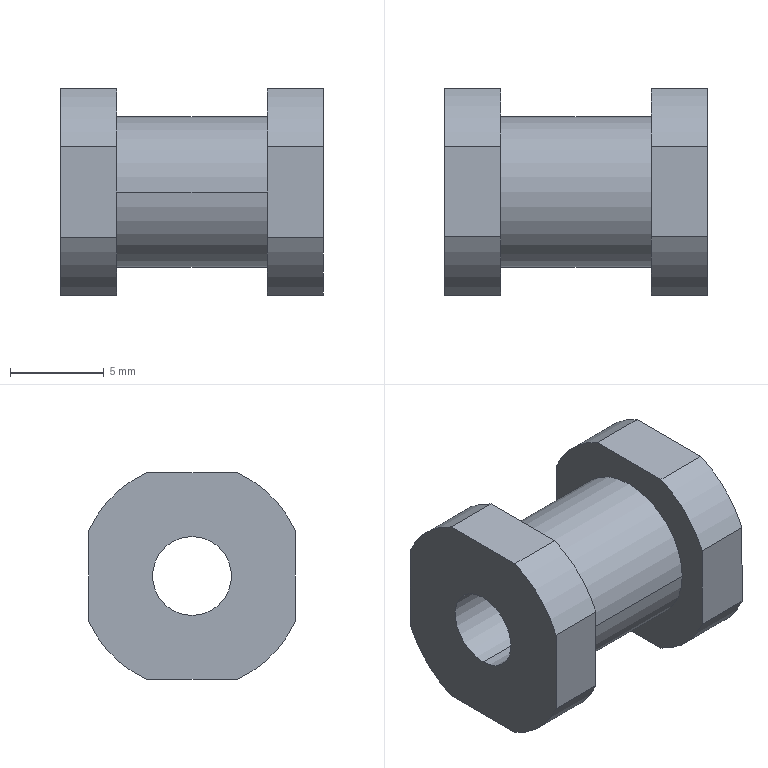Part | SolidWorks | features HoleWzd 1, ICE 1, Revolution 1 | 1 solid | 24 faces | box 14 x 11 x 11 mm | volume 848.048 mm3 | cylinder 12 | plane 12 | commonest cylinder face diameters 12 x8 4.2 x2 8 x2
STEP:
#1=CARTESIAN_POINT('',(14.,0.,-2.1));
#2=VERTEX_POINT('',#1);
#3=CARTESIAN_POINT('',(14.,0.,2.1));
#4=VERTEX_POINT('',#3);
#5=CARTESIAN_POINT('',(14.,0.,0.));
#6=DIRECTION('',(-1.,0.,0.));
#7=DIRECTION('',(0.,0.,1.));
#8=AXIS2_PLACEMENT_3D('',#5,#6,#7);
#9=CIRCLE('',#8,2.1);
#10=EDGE_CURVE('',#2,#4,#9,.T.);
#11=ORIENTED_EDGE('',*,*,#10,.F.);
#12=CARTESIAN_POINT('',(0.,0.,-2.1));
#13=VERTEX_POINT('',#12);
#14=CARTESIAN_POINT('',(0.,0.,-2.1));
#15=DIRECTION('',(-1.,0.,0.));
#16=VECTOR('',#15,1000.);
#17=LINE('',#14,#16);
#18=EDGE_CURVE('',#2,#13,#17,.T.);
#19=ORIENTED_EDGE('',*,*,#18,.T.);
#20=CARTESIAN_POINT('',(0.,0.,2.1));
#21=VERTEX_POINT('',#20);
#22=CARTESIAN_POINT('',(0.,0.,0.));
#23=DIRECTION('',(-1.,0.,0.));
#24=DIRECTION('',(0.,0.,1.));
#25=AXIS2_PLACEMENT_3D('',#22,#23,#24);
#26=CIRCLE('',#25,2.1);
#27=EDGE_CURVE('',#13,#21,#26,.T.);
#28=ORIENTED_EDGE('',*,*,#27,.T.);
#29=CARTESIAN_POINT('',(0.,0.,2.1));
#30=DIRECTION('',(-1.,0.,0.));
#31=VECTOR('',#30,1000.);
#32=LINE('',#29,#31);
#33=EDGE_CURVE('',#4,#21,#32,.T.);
#34=ORIENTED_EDGE('',*,*,#33,.F.);
#35=EDGE_LOOP('',(#11,#19,#28,#34));
#36=FACE_OUTER_BOUND('',#35,.T.);
#37=CARTESIAN_POINT('',(0.,0.,0.));
#38=DIRECTION('',(-1.,0.,0.));
#39=DIRECTION('',(0.,0.,1.));
#40=AXIS2_PLACEMENT_3D('',#37,#38,#39);
#41=CYLINDRICAL_SURFACE('',#40,2.1);
#42=ADVANCED_FACE('',(#36),#41,.F.);
#43=CARTESIAN_POINT('',(3.,4.,0.));
#44=VERTEX_POINT('',#43);
#45=CARTESIAN_POINT('',(3.,-4.,0.));
#46=VERTEX_POINT('',#45);
#47=CARTESIAN_POINT('',(3.,0.,0.));
#48=DIRECTION('',(1.,0.,0.));
#49=DIRECTION('',(0.,1.,0.));
#50=AXIS2_PLACEMENT_3D('',#47,#48,#49);
#51=CIRCLE('',#50,4.);
#52=EDGE_CURVE('',#44,#46,#51,.T.);
#53=ORIENTED_EDGE('',*,*,#52,.T.);
#54=CARTESIAN_POINT('',(11.,-4.,0.));
#55=VERTEX_POINT('',#54);
#56=CARTESIAN_POINT('',(14.,-4.,0.));
#57=DIRECTION('',(1.,0.,0.));
#58=VECTOR('',#57,1000.);
#59=LINE('',#56,#58);
#60=EDGE_CURVE('',#46,#55,#59,.T.);
#61=ORIENTED_EDGE('',*,*,#60,.T.);
#62=CARTESIAN_POINT('',(11.,4.,0.));
#63=VERTEX_POINT('',#62);
#64=CARTESIAN_POINT('',(11.,0.,0.));
#65=DIRECTION('',(1.,0.,0.));
#66=DIRECTION('',(0.,1.,0.));
#67=AXIS2_PLACEMENT_3D('',#64,#65,#66);
#68=CIRCLE('',#67,4.);
#69=EDGE_CURVE('',#63,#55,#68,.T.);
#70=ORIENTED_EDGE('',*,*,#69,.F.);
#71=CARTESIAN_POINT('',(14.,4.,0.));
#72=DIRECTION('',(1.,0.,0.));
#73=VECTOR('',#72,1000.);
#74=LINE('',#71,#73);
#75=EDGE_CURVE('',#44,#63,#74,.T.);
#76=ORIENTED_EDGE('',*,*,#75,.F.);
#77=EDGE_LOOP('',(#53,#61,#70,#76));
#78=FACE_OUTER_BOUND('',#77,.T.);
#79=CARTESIAN_POINT('',(14.,0.,0.));
#80=DIRECTION('',(1.,0.,0.));
#81=DIRECTION('',(0.,1.,0.));
#82=AXIS2_PLACEMENT_3D('',#79,#80,#81);
#83=CYLINDRICAL_SURFACE('',#82,4.);
#84=ADVANCED_FACE('',(#78),#83,.T.);
#85=CARTESIAN_POINT('',(3.,-2.398,5.5));
#86=VERTEX_POINT('',#85);
#87=CARTESIAN_POINT('',(3.,-5.5,2.398));
#88=VERTEX_POINT('',#87);
#89=CARTESIAN_POINT('',(3.,0.,0.));
#90=DIRECTION('',(1.,0.,0.));
#91=DIRECTION('',(0.,1.,0.));
#92=AXIS2_PLACEMENT_3D('',#89,#90,#91);
#93=CIRCLE('',#92,6.);
#94=EDGE_CURVE('',#86,#88,#93,.T.);
#95=ORIENTED_EDGE('',*,*,#94,.F.);
#96=CARTESIAN_POINT('',(0.,-2.398,5.5));
#97=VERTEX_POINT('',#96);
#98=CARTESIAN_POINT('',(14.,-2.398,5.5));
#99=DIRECTION('',(-1.,0.,0.));
#100=VECTOR('',#99,1000.);
#101=LINE('',#98,#100);
#102=EDGE_CURVE('',#86,#97,#101,.T.);
#103=ORIENTED_EDGE('',*,*,#102,.T.);
#104=CARTESIAN_POINT('',(0.,-5.5,2.398));
#105=VERTEX_POINT('',#104);
#106=CARTESIAN_POINT('',(0.,0.,0.));
#107=DIRECTION('',(1.,0.,0.));
#108=DIRECTION('',(0.,1.,0.));
#109=AXIS2_PLACEMENT_3D('',#106,#107,#108);
#110=CIRCLE('',#109,6.);
#111=EDGE_CURVE('',#97,#105,#110,.T.);
#112=ORIENTED_EDGE('',*,*,#111,.T.);
#113=CARTESIAN_POINT('',(14.,-5.5,2.398));
#114=DIRECTION('',(1.,0.,0.));
#115=VECTOR('',#114,1000.);
#116=LINE('',#113,#115);
#117=EDGE_CURVE('',#105,#88,#116,.T.);
#118=ORIENTED_EDGE('',*,*,#117,.T.);
#119=EDGE_LOOP('',(#95,#103,#112,#118));
#120=FACE_OUTER_BOUND('',#119,.T.);
#121=CARTESIAN_POINT('',(14.,0.,0.));
#122=DIRECTION('',(1.,0.,0.));
#123=DIRECTION('',(0.,1.,0.));
#124=AXIS2_PLACEMENT_3D('',#121,#122,#123);
#125=CYLINDRICAL_SURFACE('',#124,6.);
#126=ADVANCED_FACE('',(#120),#125,.T.);
#127=CARTESIAN_POINT('',(0.,5.5,2.398));
#128=VERTEX_POINT('',#127);
#129=CARTESIAN_POINT('',(0.,2.398,5.5));
#130=VERTEX_POINT('',#129);
#131=CARTESIAN_POINT('',(0.,0.,0.));
#132=DIRECTION('',(1.,0.,0.));
#133=DIRECTION('',(0.,1.,0.));
#134=AXIS2_PLACEMENT_3D('',#131,#132,#133);
#135=CIRCLE('',#134,6.);
#136=EDGE_CURVE('',#128,#130,#135,.T.);
#137=ORIENTED_EDGE('',*,*,#136,.T.);
#138=CARTESIAN_POINT('',(3.,2.398,5.5));
#139=VERTEX_POINT('',#138);
#140=CARTESIAN_POINT('',(14.,2.398,5.5));
#141=DIRECTION('',(1.,0.,0.));
#142=VECTOR('',#141,1000.);
#143=LINE('',#140,#142);
#144=EDGE_CURVE('',#130,#139,#143,.T.);
#145=ORIENTED_EDGE('',*,*,#144,.T.);
#146=CARTESIAN_POINT('',(3.,5.5,2.398));
#147=VERTEX_POINT('',#146);
#148=CARTESIAN_POINT('',(3.,0.,0.));
#149=DIRECTION('',(1.,0.,0.));
#150=DIRECTION('',(0.,1.,0.));
#151=AXIS2_PLACEMENT_3D('',#148,#149,#150);
#152=CIRCLE('',#151,6.);
#153=EDGE_CURVE('',#147,#139,#152,.T.);
#154=ORIENTED_EDGE('',*,*,#153,.F.);
#155=CARTESIAN_POINT('',(14.,5.5,2.398));
#156=DIRECTION('',(-1.,0.,0.));
#157=VECTOR('',#156,1000.);
#158=LINE('',#155,#157);
#159=EDGE_CURVE('',#147,#128,#158,.T.);
#160=ORIENTED_EDGE('',*,*,#159,.T.);
#161=EDGE_LOOP('',(#137,#145,#154,#160));
#162=FACE_OUTER_BOUND('',#161,.T.);
#163=CARTESIAN_POINT('',(14.,0.,0.));
#164=DIRECTION('',(1.,0.,0.));
#165=DIRECTION('',(0.,1.,0.));
#166=AXIS2_PLACEMENT_3D('',#163,#164,#165);
#167=CYLINDRICAL_SURFACE('',#166,6.);
#168=ADVANCED_FACE('',(#162),#167,.T.);
#169=CARTESIAN_POINT('',(3.,-5.5,-2.398));
#170=VERTEX_POINT('',#169);
#171=CARTESIAN_POINT('',(3.,-2.398,-5.5));
#172=VERTEX_POINT('',#171);
#173=CARTESIAN_POINT('',(3.,0.,0.));
#174=DIRECTION('',(1.,0.,0.));
#175=DIRECTION('',(0.,1.,0.));
#176=AXIS2_PLACEMENT_3D('',#173,#174,#175);
#177=CIRCLE('',#176,6.);
#178=EDGE_CURVE('',#170,#172,#177,.T.);
#179=ORIENTED_EDGE('',*,*,#178,.F.);
#180=CARTESIAN_POINT('',(0.,-5.5,-2.398));
#181=VERTEX_POINT('',#180);
#182=CARTESIAN_POINT('',(14.,-5.5,-2.398));
#183=DIRECTION('',(-1.,0.,0.));
#184=VECTOR('',#183,1000.);
#185=LINE('',#182,#184);
#186=EDGE_CURVE('',#170,#181,#185,.T.);
#187=ORIENTED_EDGE('',*,*,#186,.T.);
#188=CARTESIAN_POINT('',(0.,-2.398,-5.5));
#189=VERTEX_POINT('',#188);
#190=CARTESIAN_POINT('',(0.,0.,0.));
#191=DIRECTION('',(1.,0.,0.));
#192=DIRECTION('',(0.,1.,0.));
#193=AXIS2_PLACEMENT_3D('',#190,#191,#192);
#194=CIRCLE('',#193,6.);
#195=EDGE_CURVE('',#181,#189,#194,.T.);
#196=ORIENTED_EDGE('',*,*,#195,.T.);
#197=CARTESIAN_POINT('',(14.,-2.398,-5.5));
#198=DIRECTION('',(1.,0.,0.));
#199=VECTOR('',#198,1000.);
#200=LINE('',#197,#199);
#201=EDGE_CURVE('',#189,#172,#200,.T.);
#202=ORIENTED_EDGE('',*,*,#201,.T.);
#203=EDGE_LOOP('',(#179,#187,#196,#202));
#204=FACE_OUTER_BOUND('',#203,.T.);
#205=CARTESIAN_POINT('',(14.,0.,0.));
#206=DIRECTION('',(1.,0.,0.));
#207=DIRECTION('',(0.,1.,0.));
#208=AXIS2_PLACEMENT_3D('',#205,#206,#207);
#209=CYLINDRICAL_SURFACE('',#208,6.);
#210=ADVANCED_FACE('',(#204),#209,.T.);
#211=CARTESIAN_POINT('',(3.,2.398,-5.5));
#212=VERTEX_POINT('',#211);
#213=CARTESIAN_POINT('',(3.,5.5,-2.398));
#214=VERTEX_POINT('',#213);
#215=CARTESIAN_POINT('',(3.,0.,0.));
#216=DIRECTION('',(1.,0.,0.));
#217=DIRECTION('',(0.,1.,0.));
#218=AXIS2_PLACEMENT_3D('',#215,#216,#217);
#219=CIRCLE('',#218,6.);
#220=EDGE_CURVE('',#212,#214,#219,.T.);
#221=ORIENTED_EDGE('',*,*,#220,.F.);
#222=CARTESIAN_POINT('',(0.,2.398,-5.5));
#223=VERTEX_POINT('',#222);
#224=CARTESIAN_POINT('',(14.,2.398,-5.5));
#225=DIRECTION('',(-1.,0.,0.));
#226=VECTOR('',#225,1000.);
#227=LINE('',#224,#226);
#228=EDGE_CURVE('',#212,#223,#227,.T.);
#229=ORIENTED_EDGE('',*,*,#228,.T.);
#230=CARTESIAN_POINT('',(0.,5.5,-2.398));
#231=VERTEX_POINT('',#230);
#232=CARTESIAN_POINT('',(0.,0.,0.));
#233=DIRECTION('',(1.,0.,0.));
#234=DIRECTION('',(0.,1.,0.));
#235=AXIS2_PLACEMENT_3D('',#232,#233,#234);
#236=CIRCLE('',#235,6.);
#237=EDGE_CURVE('',#223,#231,#236,.T.);
#238=ORIENTED_EDGE('',*,*,#237,.T.);
#239=CARTESIAN_POINT('',(14.,5.5,-2.398));
#240=DIRECTION('',(1.,0.,0.));
#241=VECTOR('',#240,1000.);
#242=LINE('',#239,#241);
#243=EDGE_CURVE('',#231,#214,#242,.T.);
#244=ORIENTED_EDGE('',*,*,#243,.T.);
#245=EDGE_LOOP('',(#221,#229,#238,#244));
#246=FACE_OUTER_BOUND('',#245,.T.);
#247=CARTESIAN_POINT('',(14.,0.,0.));
#248=DIRECTION('',(1.,0.,0.));
#249=DIRECTION('',(0.,1.,0.));
#250=AXIS2_PLACEMENT_3D('',#247,#248,#249);
#251=CYLINDRICAL_SURFACE('',#250,6.);
#252=ADVANCED_FACE('',(#246),#251,.T.);
#253=ORIENTED_EDGE('',*,*,#52,.F.);
#254=CARTESIAN_POINT('',(3.,0.,0.));
#255=DIRECTION('',(1.,0.,0.));
#256=DIRECTION('',(0.,1.,0.));
#257=AXIS2_PLACEMENT_3D('',#254,#255,#256);
#258=CIRCLE('',#257,4.);
#259=EDGE_CURVE('',#46,#44,#258,.T.);
#260=ORIENTED_EDGE('',*,*,#259,.F.);
#261=EDGE_LOOP('',(#253,#260));
#262=FACE_BOUND('',#261,.T.);
#263=ORIENTED_EDGE('',*,*,#153,.T.);
#264=CARTESIAN_POINT('',(3.,6.,5.5));
#265=DIRECTION('',(0.,-1.,0.));
#266=VECTOR('',#265,1000.);
#267=LINE('',#264,#266);
#268=EDGE_CURVE('',#139,#86,#267,.T.);
#269=ORIENTED_EDGE('',*,*,#268,.T.);
#270=ORIENTED_EDGE('',*,*,#94,.T.);
#271=CARTESIAN_POINT('',(3.,-5.5,0.));
#272=DIRECTION('',(0.,0.,-1.));
#273=VECTOR('',#272,1000.);
#274=LINE('',#271,#273);
#275=EDGE_CURVE('',#88,#170,#274,.T.);
#276=ORIENTED_EDGE('',*,*,#275,.T.);
#277=ORIENTED_EDGE('',*,*,#178,.T.);
#278=CARTESIAN_POINT('',(3.,6.,-5.5));
#279=DIRECTION('',(0.,1.,0.));
#280=VECTOR('',#279,1000.);
#281=LINE('',#278,#280);
#282=EDGE_CURVE('',#172,#212,#281,.T.);
#283=ORIENTED_EDGE('',*,*,#282,.T.);
#284=ORIENTED_EDGE('',*,*,#220,.T.);
#285=CARTESIAN_POINT('',(3.,5.5,0.));
#286=DIRECTION('',(0.,0.,1.));
#287=VECTOR('',#286,1000.);
#288=LINE('',#285,#287);
#289=EDGE_CURVE('',#214,#147,#288,.T.);
#290=ORIENTED_EDGE('',*,*,#289,.T.);
#291=EDGE_LOOP('',(#263,#269,#270,#276,#277,#283,#284,#290));
#292=FACE_OUTER_BOUND('',#291,.T.);
#293=CARTESIAN_POINT('',(3.,6.,0.));
#294=DIRECTION('',(1.,0.,0.));
#295=DIRECTION('',(0.,1.,0.));
#296=AXIS2_PLACEMENT_3D('',#293,#294,#295);
#297=PLANE('',#296);
#298=ADVANCED_FACE('',(#262,#292),#297,.T.);
#299=ORIENTED_EDGE('',*,*,#69,.T.);
#300=CARTESIAN_POINT('',(11.,0.,0.));
#301=DIRECTION('',(1.,0.,0.));
#302=DIRECTION('',(0.,1.,0.));
#303=AXIS2_PLACEMENT_3D('',#300,#301,#302);
#304=CIRCLE('',#303,4.);
#305=EDGE_CURVE('',#55,#63,#304,.T.);
#306=ORIENTED_EDGE('',*,*,#305,.T.);
#307=EDGE_LOOP('',(#299,#306));
#308=FACE_BOUND('',#307,.T.);
#309=CARTESIAN_POINT('',(11.,-2.398,5.5));
#310=VERTEX_POINT('',#309);
#311=CARTESIAN_POINT('',(11.,-5.5,2.398));
#312=VERTEX_POINT('',#311);
#313=CARTESIAN_POINT('',(11.,0.,0.));
#314=DIRECTION('',(1.,0.,0.));
#315=DIRECTION('',(0.,1.,0.));
#316=AXIS2_PLACEMENT_3D('',#313,#314,#315);
#317=CIRCLE('',#316,6.);
#318=EDGE_CURVE('',#310,#312,#317,.T.);
#319=ORIENTED_EDGE('',*,*,#318,.F.);
#320=CARTESIAN_POINT('',(11.,2.398,5.5));
#321=VERTEX_POINT('',#320);
#322=CARTESIAN_POINT('',(11.,4.,5.5));
#323=DIRECTION('',(0.,1.,0.));
#324=VECTOR('',#323,1000.);
#325=LINE('',#322,#324);
#326=EDGE_CURVE('',#310,#321,#325,.T.);
#327=ORIENTED_EDGE('',*,*,#326,.T.);
#328=CARTESIAN_POINT('',(11.,5.5,2.398));
#329=VERTEX_POINT('',#328);
#330=CARTESIAN_POINT('',(11.,0.,0.));
#331=DIRECTION('',(1.,0.,0.));
#332=DIRECTION('',(0.,1.,0.));
#333=AXIS2_PLACEMENT_3D('',#330,#331,#332);
#334=CIRCLE('',#333,6.);
#335=EDGE_CURVE('',#329,#321,#334,.T.);
#336=ORIENTED_EDGE('',*,*,#335,.F.);
#337=CARTESIAN_POINT('',(11.,5.5,-2.398));
#338=VERTEX_POINT('',#337);
#339=CARTESIAN_POINT('',(11.,5.5,0.));
#340=DIRECTION('',(0.,0.,-1.));
#341=VECTOR('',#340,1000.);
#342=LINE('',#339,#341);
#343=EDGE_CURVE('',#329,#338,#342,.T.);
#344=ORIENTED_EDGE('',*,*,#343,.T.);
#345=CARTESIAN_POINT('',(11.,2.398,-5.5));
#346=VERTEX_POINT('',#345);
#347=CARTESIAN_POINT('',(11.,0.,0.));
#348=DIRECTION('',(1.,0.,0.));
#349=DIRECTION('',(0.,1.,0.));
#350=AXIS2_PLACEMENT_3D('',#347,#348,#349);
#351=CIRCLE('',#350,6.);
#352=EDGE_CURVE('',#346,#338,#351,.T.);
#353=ORIENTED_EDGE('',*,*,#352,.F.);
#354=CARTESIAN_POINT('',(11.,-2.398,-5.5));
#355=VERTEX_POINT('',#354);
#356=CARTESIAN_POINT('',(11.,4.,-5.5));
#357=DIRECTION('',(0.,-1.,0.));
#358=VECTOR('',#357,1000.);
#359=LINE('',#356,#358);
#360=EDGE_CURVE('',#346,#355,#359,.T.);
#361=ORIENTED_EDGE('',*,*,#360,.T.);
#362=CARTESIAN_POINT('',(11.,-5.5,-2.398));
#363=VERTEX_POINT('',#362);
#364=CARTESIAN_POINT('',(11.,0.,0.));
#365=DIRECTION('',(1.,0.,0.));
#366=DIRECTION('',(0.,1.,0.));
#367=AXIS2_PLACEMENT_3D('',#364,#365,#366);
#368=CIRCLE('',#367,6.);
#369=EDGE_CURVE('',#363,#355,#368,.T.);
#370=ORIENTED_EDGE('',*,*,#369,.F.);
#371=CARTESIAN_POINT('',(11.,-5.5,0.));
#372=DIRECTION('',(0.,0.,1.));
#373=VECTOR('',#372,1000.);
#374=LINE('',#371,#373);
#375=EDGE_CURVE('',#363,#312,#374,.T.);
#376=ORIENTED_EDGE('',*,*,#375,.T.);
#377=EDGE_LOOP('',(#319,#327,#336,#344,#353,#361,#370,#376));
#378=FACE_OUTER_BOUND('',#377,.T.);
#379=CARTESIAN_POINT('',(11.,4.,0.));
#380=DIRECTION('',(-1.,0.,0.));
#381=DIRECTION('',(0.,-1.,0.));
#382=AXIS2_PLACEMENT_3D('',#379,#380,#381);
#383=PLANE('',#382);
#384=ADVANCED_FACE('',(#308,#378),#383,.T.);
#385=CARTESIAN_POINT('',(14.,-2.398,5.5));
#386=VERTEX_POINT('',#385);
#387=CARTESIAN_POINT('',(14.,-5.5,2.398));
#388=VERTEX_POINT('',#387);
#389=CARTESIAN_POINT('',(14.,0.,0.));
#390=DIRECTION('',(1.,0.,0.));
#391=DIRECTION('',(0.,1.,0.));
#392=AXIS2_PLACEMENT_3D('',#389,#390,#391);
#393=CIRCLE('',#392,6.);
#394=EDGE_CURVE('',#386,#388,#393,.T.);
#395=ORIENTED_EDGE('',*,*,#394,.F.);
#396=CARTESIAN_POINT('',(14.,-2.398,5.5));
#397=DIRECTION('',(-1.,0.,0.));
#398=VECTOR('',#397,1000.);
#399=LINE('',#396,#398);
#400=EDGE_CURVE('',#386,#310,#399,.T.);
#401=ORIENTED_EDGE('',*,*,#400,.T.);
#402=ORIENTED_EDGE('',*,*,#318,.T.);
#403=CARTESIAN_POINT('',(14.,-5.5,2.398));
#404=DIRECTION('',(1.,0.,0.));
#405=VECTOR('',#404,1000.);
#406=LINE('',#403,#405);
#407=EDGE_CURVE('',#312,#388,#406,.T.);
#408=ORIENTED_EDGE('',*,*,#407,.T.);
#409=EDGE_LOOP('',(#395,#401,#402,#408));
#410=FACE_OUTER_BOUND('',#409,.T.);
#411=CARTESIAN_POINT('',(14.,0.,0.));
#412=DIRECTION('',(1.,0.,0.));
#413=DIRECTION('',(0.,1.,0.));
#414=AXIS2_PLACEMENT_3D('',#411,#412,#413);
#415=CYLINDRICAL_SURFACE('',#414,6.);
#416=ADVANCED_FACE('',(#410),#415,.T.);
#417=ORIENTED_EDGE('',*,*,#335,.T.);
#418=CARTESIAN_POINT('',(14.,2.398,5.5));
#419=VERTEX_POINT('',#418);
#420=CARTESIAN_POINT('',(14.,2.398,5.5));
#421=DIRECTION('',(1.,0.,0.));
#422=VECTOR('',#421,1000.);
#423=LINE('',#420,#422);
#424=EDGE_CURVE('',#321,#419,#423,.T.);
#425=ORIENTED_EDGE('',*,*,#424,.T.);
#426=CARTESIAN_POINT('',(14.,5.5,2.398));
#427=VERTEX_POINT('',#426);
#428=CARTESIAN_POINT('',(14.,0.,0.));
#429=DIRECTION('',(1.,0.,0.));
#430=DIRECTION('',(0.,1.,0.));
#431=AXIS2_PLACEMENT_3D('',#428,#429,#430);
#432=CIRCLE('',#431,6.);
#433=EDGE_CURVE('',#427,#419,#432,.T.);
#434=ORIENTED_EDGE('',*,*,#433,.F.);
#435=CARTESIAN_POINT('',(14.,5.5,2.398));
#436=DIRECTION('',(-1.,0.,0.));
#437=VECTOR('',#436,1000.);
#438=LINE('',#435,#437);
#439=EDGE_CURVE('',#427,#329,#438,.T.);
#440=ORIENTED_EDGE('',*,*,#439,.T.);
#441=EDGE_LOOP('',(#417,#425,#434,#440));
#442=FACE_OUTER_BOUND('',#441,.T.);
#443=CARTESIAN_POINT('',(14.,0.,0.));
#444=DIRECTION('',(1.,0.,0.));
#445=DIRECTION('',(0.,1.,0.));
#446=AXIS2_PLACEMENT_3D('',#443,#444,#445);
#447=CYLINDRICAL_SURFACE('',#446,6.);
#448=ADVANCED_FACE('',(#442),#447,.T.);
#449=CARTESIAN_POINT('',(14.,-5.5,-2.398));
#450=VERTEX_POINT('',#449);
#451=CARTESIAN_POINT('',(14.,-2.398,-5.5));
#452=VERTEX_POINT('',#451);
#453=CARTESIAN_POINT('',(14.,0.,0.));
#454=DIRECTION('',(1.,0.,0.));
#455=DIRECTION('',(0.,1.,0.));
#456=AXIS2_PLACEMENT_3D('',#453,#454,#455);
#457=CIRCLE('',#456,6.);
#458=EDGE_CURVE('',#450,#452,#457,.T.);
#459=ORIENTED_EDGE('',*,*,#458,.F.);
#460=CARTESIAN_POINT('',(14.,-5.5,-2.398));
#461=DIRECTION('',(-1.,0.,0.));
#462=VECTOR('',#461,1000.);
#463=LINE('',#460,#462);
#464=EDGE_CURVE('',#450,#363,#463,.T.);
#465=ORIENTED_EDGE('',*,*,#464,.T.);
#466=ORIENTED_EDGE('',*,*,#369,.T.);
#467=CARTESIAN_POINT('',(14.,-2.398,-5.5));
#468=DIRECTION('',(1.,0.,0.));
#469=VECTOR('',#468,1000.);
#470=LINE('',#467,#469);
#471=EDGE_CURVE('',#355,#452,#470,.T.);
#472=ORIENTED_EDGE('',*,*,#471,.T.);
#473=EDGE_LOOP('',(#459,#465,#466,#472));
#474=FACE_OUTER_BOUND('',#473,.T.);
#475=CARTESIAN_POINT('',(14.,0.,0.));
#476=DIRECTION('',(1.,0.,0.));
#477=DIRECTION('',(0.,1.,0.));
#478=AXIS2_PLACEMENT_3D('',#475,#476,#477);
#479=CYLINDRICAL_SURFACE('',#478,6.);
#480=ADVANCED_FACE('',(#474),#479,.T.);
#481=CARTESIAN_POINT('',(14.,2.398,-5.5));
#482=VERTEX_POINT('',#481);
#483=CARTESIAN_POINT('',(14.,5.5,-2.398));
#484=VERTEX_POINT('',#483);
#485=CARTESIAN_POINT('',(14.,0.,0.));
#486=DIRECTION('',(1.,0.,0.));
#487=DIRECTION('',(0.,1.,0.));
#488=AXIS2_PLACEMENT_3D('',#485,#486,#487);
#489=CIRCLE('',#488,6.);
#490=EDGE_CURVE('',#482,#484,#489,.T.);
#491=ORIENTED_EDGE('',*,*,#490,.F.);
#492=CARTESIAN_POINT('',(14.,2.398,-5.5));
#493=DIRECTION('',(-1.,0.,0.));
#494=VECTOR('',#493,1000.);
#495=LINE('',#492,#494);
#496=EDGE_CURVE('',#482,#346,#495,.T.);
#497=ORIENTED_EDGE('',*,*,#496,.T.);
#498=ORIENTED_EDGE('',*,*,#352,.T.);
#499=CARTESIAN_POINT('',(14.,5.5,-2.398));
#500=DIRECTION('',(1.,0.,0.));
#501=VECTOR('',#500,1000.);
#502=LINE('',#499,#501);
#503=EDGE_CURVE('',#338,#484,#502,.T.);
#504=ORIENTED_EDGE('',*,*,#503,.T.);
#505=EDGE_LOOP('',(#491,#497,#498,#504));
#506=FACE_OUTER_BOUND('',#505,.T.);
#507=CARTESIAN_POINT('',(14.,0.,0.));
#508=DIRECTION('',(1.,0.,0.));
#509=DIRECTION('',(0.,1.,0.));
#510=AXIS2_PLACEMENT_3D('',#507,#508,#509);
#511=CYLINDRICAL_SURFACE('',#510,6.);
#512=ADVANCED_FACE('',(#506),#511,.T.);
#513=CARTESIAN_POINT('',(14.,0.,0.));
#514=DIRECTION('',(-1.,0.,0.));
#515=DIRECTION('',(0.,0.,1.));
#516=AXIS2_PLACEMENT_3D('',#513,#514,#515);
#517=CIRCLE('',#516,2.1);
#518=EDGE_CURVE('',#4,#2,#517,.T.);
#519=ORIENTED_EDGE('',*,*,#518,.T.);
#520=ORIENTED_EDGE('',*,*,#10,.T.);
#521=EDGE_LOOP('',(#519,#520));
#522=FACE_BOUND('',#521,.T.);
#523=ORIENTED_EDGE('',*,*,#433,.T.);
#524=CARTESIAN_POINT('',(14.,-5.5,5.5));
#525=DIRECTION('',(0.,1.,0.));
#526=VECTOR('',#525,1000.);
#527=LINE('',#524,#526);
#528=EDGE_CURVE('',#386,#419,#527,.T.);
#529=ORIENTED_EDGE('',*,*,#528,.F.);
#530=ORIENTED_EDGE('',*,*,#394,.T.);
#531=CARTESIAN_POINT('',(14.,-5.5,-5.5));
#532=DIRECTION('',(0.,0.,1.));
#533=VECTOR('',#532,1000.);
#534=LINE('',#531,#533);
#535=EDGE_CURVE('',#450,#388,#534,.T.);
#536=ORIENTED_EDGE('',*,*,#535,.F.);
#537=ORIENTED_EDGE('',*,*,#458,.T.);
#538=CARTESIAN_POINT('',(14.,-5.5,-5.5));
#539=DIRECTION('',(0.,-1.,0.));
#540=VECTOR('',#539,1000.);
#541=LINE('',#538,#540);
#542=EDGE_CURVE('',#482,#452,#541,.T.);
#543=ORIENTED_EDGE('',*,*,#542,.F.);
#544=ORIENTED_EDGE('',*,*,#490,.T.);
#545=CARTESIAN_POINT('',(14.,5.5,-5.5));
#546=DIRECTION('',(0.,0.,-1.));
#547=VECTOR('',#546,1000.);
#548=LINE('',#545,#547);
#549=EDGE_CURVE('',#427,#484,#548,.T.);
#550=ORIENTED_EDGE('',*,*,#549,.F.);
#551=EDGE_LOOP('',(#523,#529,#530,#536,#537,#543,#544,#550));
#552=FACE_OUTER_BOUND('',#551,.T.);
#553=CARTESIAN_POINT('',(14.,6.,0.));
#554=DIRECTION('',(1.,0.,0.));
#555=DIRECTION('',(0.,1.,0.));
#556=AXIS2_PLACEMENT_3D('',#553,#554,#555);
#557=PLANE('',#556);
#558=ADVANCED_FACE('',(#522,#552),#557,.T.);
#559=CARTESIAN_POINT('',(0.,0.,0.));
#560=DIRECTION('',(-1.,0.,0.));
#561=DIRECTION('',(0.,0.,1.));
#562=AXIS2_PLACEMENT_3D('',#559,#560,#561);
#563=CIRCLE('',#562,2.1);
#564=EDGE_CURVE('',#21,#13,#563,.T.);
#565=ORIENTED_EDGE('',*,*,#564,.F.);
#566=ORIENTED_EDGE('',*,*,#27,.F.);
#567=EDGE_LOOP('',(#565,#566));
#568=FACE_BOUND('',#567,.T.);
#569=ORIENTED_EDGE('',*,*,#111,.F.);
#570=CARTESIAN_POINT('',(0.,6.,5.5));
#571=DIRECTION('',(0.,1.,0.));
#572=VECTOR('',#571,1000.);
#573=LINE('',#570,#572);
#574=EDGE_CURVE('',#97,#130,#573,.T.);
#575=ORIENTED_EDGE('',*,*,#574,.T.);
#576=ORIENTED_EDGE('',*,*,#136,.F.);
#577=CARTESIAN_POINT('',(0.,5.5,0.));
#578=DIRECTION('',(0.,0.,-1.));
#579=VECTOR('',#578,1000.);
#580=LINE('',#577,#579);
#581=EDGE_CURVE('',#128,#231,#580,.T.);
#582=ORIENTED_EDGE('',*,*,#581,.T.);
#583=ORIENTED_EDGE('',*,*,#237,.F.);
#584=CARTESIAN_POINT('',(0.,6.,-5.5));
#585=DIRECTION('',(0.,-1.,0.));
#586=VECTOR('',#585,1000.);
#587=LINE('',#584,#586);
#588=EDGE_CURVE('',#223,#189,#587,.T.);
#589=ORIENTED_EDGE('',*,*,#588,.T.);
#590=ORIENTED_EDGE('',*,*,#195,.F.);
#591=CARTESIAN_POINT('',(0.,-5.5,0.));
#592=DIRECTION('',(0.,0.,1.));
#593=VECTOR('',#592,1000.);
#594=LINE('',#591,#593);
#595=EDGE_CURVE('',#181,#105,#594,.T.);
#596=ORIENTED_EDGE('',*,*,#595,.T.);
#597=EDGE_LOOP('',(#569,#575,#576,#582,#583,#589,#590,#596));
#598=FACE_OUTER_BOUND('',#597,.T.);
#599=CARTESIAN_POINT('',(0.,6.,0.));
#600=DIRECTION('',(-1.,0.,0.));
#601=DIRECTION('',(0.,-1.,0.));
#602=AXIS2_PLACEMENT_3D('',#599,#600,#601);
#603=PLANE('',#602);
#604=ADVANCED_FACE('',(#568,#598),#603,.T.);
#605=ORIENTED_EDGE('',*,*,#60,.F.);
#606=ORIENTED_EDGE('',*,*,#259,.T.);
#607=ORIENTED_EDGE('',*,*,#75,.T.);
#608=ORIENTED_EDGE('',*,*,#305,.F.);
#609=EDGE_LOOP('',(#605,#606,#607,#608));
#610=FACE_OUTER_BOUND('',#609,.T.);
#611=CARTESIAN_POINT('',(14.,0.,0.));
#612=DIRECTION('',(1.,0.,0.));
#613=DIRECTION('',(0.,1.,0.));
#614=AXIS2_PLACEMENT_3D('',#611,#612,#613);
#615=CYLINDRICAL_SURFACE('',#614,4.);
#616=ADVANCED_FACE('',(#610),#615,.T.);
#617=ORIENTED_EDGE('',*,*,#18,.F.);
#618=ORIENTED_EDGE('',*,*,#518,.F.);
#619=ORIENTED_EDGE('',*,*,#33,.T.);
#620=ORIENTED_EDGE('',*,*,#564,.T.);
#621=EDGE_LOOP('',(#617,#618,#619,#620));
#622=FACE_OUTER_BOUND('',#621,.T.);
#623=CARTESIAN_POINT('',(0.,0.,0.));
#624=DIRECTION('',(-1.,0.,0.));
#625=DIRECTION('',(0.,0.,1.));
#626=AXIS2_PLACEMENT_3D('',#623,#624,#625);
#627=CYLINDRICAL_SURFACE('',#626,2.1);
#628=ADVANCED_FACE('',(#622),#627,.F.);
#629=ORIENTED_EDGE('',*,*,#289,.F.);
#630=ORIENTED_EDGE('',*,*,#243,.F.);
#631=ORIENTED_EDGE('',*,*,#581,.F.);
#632=ORIENTED_EDGE('',*,*,#159,.F.);
#633=EDGE_LOOP('',(#629,#630,#631,#632));
#634=FACE_OUTER_BOUND('',#633,.T.);
#635=CARTESIAN_POINT('',(14.,5.5,-5.5));
#636=DIRECTION('',(0.,1.,0.));
#637=DIRECTION('',(-1.,0.,0.));
#638=AXIS2_PLACEMENT_3D('',#635,#636,#637);
#639=PLANE('',#638);
#640=ADVANCED_FACE('',(#634),#639,.T.);
#641=ORIENTED_EDGE('',*,*,#282,.F.);
#642=ORIENTED_EDGE('',*,*,#201,.F.);
#643=ORIENTED_EDGE('',*,*,#588,.F.);
#644=ORIENTED_EDGE('',*,*,#228,.F.);
#645=EDGE_LOOP('',(#641,#642,#643,#644));
#646=FACE_OUTER_BOUND('',#645,.T.);
#647=CARTESIAN_POINT('',(14.,-5.5,-5.5));
#648=DIRECTION('',(0.,0.,-1.));
#649=DIRECTION('',(-1.,0.,0.));
#650=AXIS2_PLACEMENT_3D('',#647,#648,#649);
#651=PLANE('',#650);
#652=ADVANCED_FACE('',(#646),#651,.T.);
#653=ORIENTED_EDGE('',*,*,#275,.F.);
#654=ORIENTED_EDGE('',*,*,#117,.F.);
#655=ORIENTED_EDGE('',*,*,#595,.F.);
#656=ORIENTED_EDGE('',*,*,#186,.F.);
#657=EDGE_LOOP('',(#653,#654,#655,#656));
#658=FACE_OUTER_BOUND('',#657,.T.);
#659=CARTESIAN_POINT('',(14.,-5.5,-5.5));
#660=DIRECTION('',(0.,-1.,0.));
#661=DIRECTION('',(1.,0.,0.));
#662=AXIS2_PLACEMENT_3D('',#659,#660,#661);
#663=PLANE('',#662);
#664=ADVANCED_FACE('',(#658),#663,.T.);
#665=ORIENTED_EDGE('',*,*,#268,.F.);
#666=ORIENTED_EDGE('',*,*,#144,.F.);
#667=ORIENTED_EDGE('',*,*,#574,.F.);
#668=ORIENTED_EDGE('',*,*,#102,.F.);
#669=EDGE_LOOP('',(#665,#666,#667,#668));
#670=FACE_OUTER_BOUND('',#669,.T.);
#671=CARTESIAN_POINT('',(14.,-5.5,5.5));
#672=DIRECTION('',(0.,0.,1.));
#673=DIRECTION('',(1.,0.,0.));
#674=AXIS2_PLACEMENT_3D('',#671,#672,#673);
#675=PLANE('',#674);
#676=ADVANCED_FACE('',(#670),#675,.T.);
#677=ORIENTED_EDGE('',*,*,#549,.T.);
#678=ORIENTED_EDGE('',*,*,#503,.F.);
#679=ORIENTED_EDGE('',*,*,#343,.F.);
#680=ORIENTED_EDGE('',*,*,#439,.F.);
#681=EDGE_LOOP('',(#677,#678,#679,#680));
#682=FACE_OUTER_BOUND('',#681,.T.);
#683=CARTESIAN_POINT('',(14.,5.5,-5.5));
#684=DIRECTION('',(0.,1.,0.));
#685=DIRECTION('',(-1.,0.,0.));
#686=AXIS2_PLACEMENT_3D('',#683,#684,#685);
#687=PLANE('',#686);
#688=ADVANCED_FACE('',(#682),#687,.T.);
#689=ORIENTED_EDGE('',*,*,#542,.T.);
#690=ORIENTED_EDGE('',*,*,#471,.F.);
#691=ORIENTED_EDGE('',*,*,#360,.F.);
#692=ORIENTED_EDGE('',*,*,#496,.F.);
#693=EDGE_LOOP('',(#689,#690,#691,#692));
#694=FACE_OUTER_BOUND('',#693,.T.);
#695=CARTESIAN_POINT('',(14.,-5.5,-5.5));
#696=DIRECTION('',(0.,0.,-1.));
#697=DIRECTION('',(-1.,0.,0.));
#698=AXIS2_PLACEMENT_3D('',#695,#696,#697);
#699=PLANE('',#698);
#700=ADVANCED_FACE('',(#694),#699,.T.);
#701=ORIENTED_EDGE('',*,*,#535,.T.);
#702=ORIENTED_EDGE('',*,*,#407,.F.);
#703=ORIENTED_EDGE('',*,*,#375,.F.);
#704=ORIENTED_EDGE('',*,*,#464,.F.);
#705=EDGE_LOOP('',(#701,#702,#703,#704));
#706=FACE_OUTER_BOUND('',#705,.T.);
#707=CARTESIAN_POINT('',(14.,-5.5,-5.5));
#708=DIRECTION('',(0.,-1.,0.));
#709=DIRECTION('',(1.,0.,0.));
#710=AXIS2_PLACEMENT_3D('',#707,#708,#709);
#711=PLANE('',#710);
#712=ADVANCED_FACE('',(#706),#711,.T.);
#713=ORIENTED_EDGE('',*,*,#528,.T.);
#714=ORIENTED_EDGE('',*,*,#424,.F.);
#715=ORIENTED_EDGE('',*,*,#326,.F.);
#716=ORIENTED_EDGE('',*,*,#400,.F.);
#717=EDGE_LOOP('',(#713,#714,#715,#716));
#718=FACE_OUTER_BOUND('',#717,.T.);
#719=CARTESIAN_POINT('',(14.,-5.5,5.5));
#720=DIRECTION('',(0.,0.,1.));
#721=DIRECTION('',(1.,0.,0.));
#722=AXIS2_PLACEMENT_3D('',#719,#720,#721);
#723=PLANE('',#722);
#724=ADVANCED_FACE('',(#718),#723,.T.);
#725=CLOSED_SHELL('',(#42,#84,#126,#168,#210,#252,#298,#384,#416,#448,#480,#512,#558,#604,#616,#628,#640,#652,#664,#676,#688,#700,#712,#724));
#726=MANIFOLD_SOLID_BREP('',#725);
#727=CARTESIAN_POINT('',(0.,0.,0.));
#728=DIRECTION('',(0.,0.,1.));
#729=DIRECTION('',(1.,0.,0.));
#730=AXIS2_PLACEMENT_3D('',#727,#728,#729);
#731=(LENGTH_UNIT()NAMED_UNIT(*)SI_UNIT(.MILLI.,.METRE.));
#732=UNCERTAINTY_MEASURE_WITH_UNIT(LENGTH_MEASURE(0.00001),#731,'','');
#733=(NAMED_UNIT(*)PLANE_ANGLE_UNIT()SI_UNIT($,.RADIAN.));
#734=(NAMED_UNIT(*)SI_UNIT($,.STERADIAN.)SOLID_ANGLE_UNIT());
#735=(GEOMETRIC_REPRESENTATION_CONTEXT(3)GLOBAL_UNCERTAINTY_ASSIGNED_CONTEXT((#732))GLOBAL_UNIT_ASSIGNED_CONTEXT((#731,#733,#734))REPRESENTATION_CONTEXT('',''));
#736=ADVANCED_BREP_SHAPE_REPRESENTATION('',(#726,#730),#735);